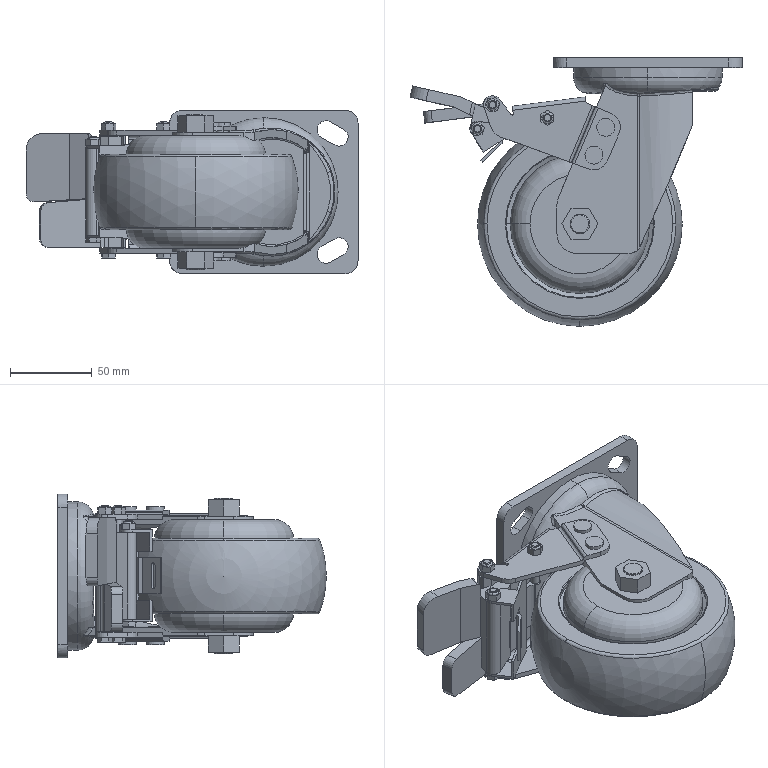Part | SolidWorks | 15 solids | 445 faces | box 202.75 x 164 x 100 mm | volume 915324 mm3 | plane 215 | cylinder 156 | torus 30 | spline 23 | cone 19 | sphere 2 | commonest cylinder face diameters 5 x34 11 x25 8 x24 4 x11 10 x8 20 x8